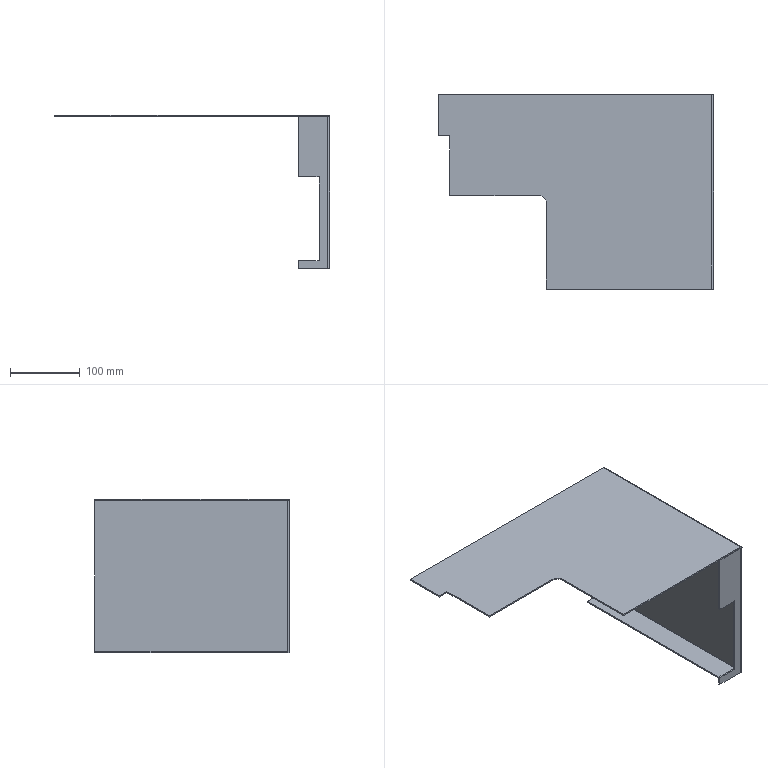Part | STEP file | TX-003 | 1 solid | 33 faces | box 395 x 279 x 220.81 mm | volume 327084 mm3 | plane 26 | cylinder 7 | commonest cylinder face diameters 1 x3 5 x3 20 x1
STEP:
#1=CARTESIAN_POINT('',(-54.654,279.925,0.));
#2=VERTEX_POINT('',#1);
#3=CARTESIAN_POINT('',(-44.654,269.925,0.));
#4=VERTEX_POINT('',#3);
#5=CARTESIAN_POINT('',(-54.654,269.925,0.));
#6=DIRECTION('',(0.,0.,-1.));
#7=DIRECTION('',(-1.,0.,0.));
#8=AXIS2_PLACEMENT_3D('',#5,#6,#7);
#9=CIRCLE('',#8,10.);
#10=EDGE_CURVE('',#2,#4,#9,.T.);
#11=ORIENTED_EDGE('',*,*,#10,.T.);
#12=CARTESIAN_POINT('',(-44.654,145.925,0.));
#13=VERTEX_POINT('',#12);
#14=CARTESIAN_POINT('',(-44.654,0.,0.));
#15=DIRECTION('',(0.,-1.,0.));
#16=VECTOR('',#15,1000.);
#17=LINE('',#14,#16);
#18=EDGE_CURVE('',#4,#13,#17,.T.);
#19=ORIENTED_EDGE('',*,*,#18,.T.);
#20=CARTESIAN_POINT('',(192.846,145.925,0.));
#21=VERTEX_POINT('',#20);
#22=CARTESIAN_POINT('',(0.,145.925,0.));
#23=DIRECTION('',(1.,0.,0.));
#24=VECTOR('',#23,1000.);
#25=LINE('',#22,#24);
#26=EDGE_CURVE('',#13,#21,#25,.T.);
#27=ORIENTED_EDGE('',*,*,#26,.T.);
#28=CARTESIAN_POINT('',(192.846,424.925,0.));
#29=VERTEX_POINT('',#28);
#30=CARTESIAN_POINT('',(192.846,0.,0.));
#31=DIRECTION('',(0.,1.,0.));
#32=VECTOR('',#31,1000.);
#33=LINE('',#30,#32);
#34=EDGE_CURVE('',#21,#29,#33,.T.);
#35=ORIENTED_EDGE('',*,*,#34,.T.);
#36=CARTESIAN_POINT('',(-199.654,424.925,0.));
#37=VERTEX_POINT('',#36);
#38=CARTESIAN_POINT('',(0.,424.925,0.));
#39=DIRECTION('',(-1.,0.,0.));
#40=VECTOR('',#39,1000.);
#41=LINE('',#38,#40);
#42=EDGE_CURVE('',#29,#37,#41,.T.);
#43=ORIENTED_EDGE('',*,*,#42,.T.);
#44=CARTESIAN_POINT('',(-199.654,365.925,0.));
#45=VERTEX_POINT('',#44);
#46=CARTESIAN_POINT('',(-199.654,0.,0.));
#47=DIRECTION('',(0.,-1.,0.));
#48=VECTOR('',#47,1000.);
#49=LINE('',#46,#48);
#50=EDGE_CURVE('',#37,#45,#49,.T.);
#51=ORIENTED_EDGE('',*,*,#50,.T.);
#52=CARTESIAN_POINT('',(-183.654,365.925,0.));
#53=VERTEX_POINT('',#52);
#54=CARTESIAN_POINT('',(0.,365.925,0.));
#55=DIRECTION('',(1.,0.,0.));
#56=VECTOR('',#55,1000.);
#57=LINE('',#54,#56);
#58=EDGE_CURVE('',#45,#53,#57,.T.);
#59=ORIENTED_EDGE('',*,*,#58,.T.);
#60=CARTESIAN_POINT('',(-183.654,279.925,0.));
#61=VERTEX_POINT('',#60);
#62=CARTESIAN_POINT('',(-183.654,0.,0.));
#63=DIRECTION('',(0.,-1.,0.));
#64=VECTOR('',#63,1000.);
#65=LINE('',#62,#64);
#66=EDGE_CURVE('',#53,#61,#65,.T.);
#67=ORIENTED_EDGE('',*,*,#66,.T.);
#68=CARTESIAN_POINT('',(0.,279.925,0.));
#69=DIRECTION('',(1.,0.,0.));
#70=VECTOR('',#69,1000.);
#71=LINE('',#68,#70);
#72=EDGE_CURVE('',#61,#2,#71,.T.);
#73=ORIENTED_EDGE('',*,*,#72,.T.);
#74=EDGE_LOOP('',(#11,#19,#27,#35,#43,#51,#59,#67,#73));
#75=FACE_OUTER_BOUND('',#74,.T.);
#76=CARTESIAN_POINT('',(0.,0.,0.));
#77=DIRECTION('',(0.,0.,1.));
#78=DIRECTION('',(1.,0.,0.));
#79=AXIS2_PLACEMENT_3D('',#76,#77,#78);
#80=PLANE('',#79);
#81=ADVANCED_FACE('',(#75),#80,.T.);
#82=CARTESIAN_POINT('',(-44.654,269.925,-2.));
#83=VERTEX_POINT('',#82);
#84=CARTESIAN_POINT('',(-44.654,145.925,-2.));
#85=VERTEX_POINT('',#84);
#86=CARTESIAN_POINT('',(-44.654,279.925,-2.));
#87=DIRECTION('',(0.,-1.,0.));
#88=VECTOR('',#87,1000.);
#89=LINE('',#86,#88);
#90=EDGE_CURVE('',#83,#85,#89,.T.);
#91=ORIENTED_EDGE('',*,*,#90,.T.);
#92=CARTESIAN_POINT('',(-44.654,145.925,-2.));
#93=DIRECTION('',(0.,0.,1.));
#94=VECTOR('',#93,1000.);
#95=LINE('',#92,#94);
#96=EDGE_CURVE('',#85,#13,#95,.T.);
#97=ORIENTED_EDGE('',*,*,#96,.T.);
#98=ORIENTED_EDGE('',*,*,#18,.F.);
#99=CARTESIAN_POINT('',(-44.654,269.925,-2.));
#100=DIRECTION('',(0.,0.,-1.));
#101=VECTOR('',#100,1000.);
#102=LINE('',#99,#101);
#103=EDGE_CURVE('',#4,#83,#102,.T.);
#104=ORIENTED_EDGE('',*,*,#103,.T.);
#105=EDGE_LOOP('',(#91,#97,#98,#104));
#106=FACE_OUTER_BOUND('',#105,.T.);
#107=CARTESIAN_POINT('',(-44.654,279.925,-2.));
#108=DIRECTION('',(-1.,0.,0.));
#109=DIRECTION('',(0.,0.,1.));
#110=AXIS2_PLACEMENT_3D('',#107,#108,#109);
#111=PLANE('',#110);
#112=ADVANCED_FACE('',(#106),#111,.T.);
#113=ORIENTED_EDGE('',*,*,#103,.F.);
#114=ORIENTED_EDGE('',*,*,#10,.F.);
#115=CARTESIAN_POINT('',(-54.654,279.925,-2.));
#116=VERTEX_POINT('',#115);
#117=CARTESIAN_POINT('',(-54.654,279.925,-2.));
#118=DIRECTION('',(0.,0.,1.));
#119=VECTOR('',#118,1000.);
#120=LINE('',#117,#119);
#121=EDGE_CURVE('',#116,#2,#120,.T.);
#122=ORIENTED_EDGE('',*,*,#121,.F.);
#123=CARTESIAN_POINT('',(-54.654,269.925,-2.));
#124=DIRECTION('',(0.,0.,1.));
#125=DIRECTION('',(-1.,0.,0.));
#126=AXIS2_PLACEMENT_3D('',#123,#124,#125);
#127=CIRCLE('',#126,10.);
#128=EDGE_CURVE('',#83,#116,#127,.T.);
#129=ORIENTED_EDGE('',*,*,#128,.F.);
#130=EDGE_LOOP('',(#113,#114,#122,#129));
#131=FACE_OUTER_BOUND('',#130,.T.);
#132=CARTESIAN_POINT('',(-54.654,269.925,-2.));
#133=DIRECTION('',(0.,0.,-1.));
#134=DIRECTION('',(-1.,0.,0.));
#135=AXIS2_PLACEMENT_3D('',#132,#133,#134);
#136=CYLINDRICAL_SURFACE('',#135,10.);
#137=ADVANCED_FACE('',(#131),#136,.F.);
#138=ORIENTED_EDGE('',*,*,#72,.F.);
#139=CARTESIAN_POINT('',(-183.654,279.925,-2.));
#140=VERTEX_POINT('',#139);
#141=CARTESIAN_POINT('',(-183.654,279.925,-2.));
#142=DIRECTION('',(0.,0.,-1.));
#143=VECTOR('',#142,1000.);
#144=LINE('',#141,#143);
#145=EDGE_CURVE('',#61,#140,#144,.T.);
#146=ORIENTED_EDGE('',*,*,#145,.T.);
#147=CARTESIAN_POINT('',(-183.654,279.925,-2.));
#148=DIRECTION('',(1.,0.,0.));
#149=VECTOR('',#148,1000.);
#150=LINE('',#147,#149);
#151=EDGE_CURVE('',#140,#116,#150,.T.);
#152=ORIENTED_EDGE('',*,*,#151,.T.);
#153=ORIENTED_EDGE('',*,*,#121,.T.);
#154=EDGE_LOOP('',(#138,#146,#152,#153));
#155=FACE_OUTER_BOUND('',#154,.T.);
#156=CARTESIAN_POINT('',(-183.654,279.925,-2.));
#157=DIRECTION('',(0.,-1.,0.));
#158=DIRECTION('',(0.,0.,-1.));
#159=AXIS2_PLACEMENT_3D('',#156,#157,#158);
#160=PLANE('',#159);
#161=ADVANCED_FACE('',(#155),#160,.T.);
#162=CARTESIAN_POINT('',(-183.654,365.925,-2.));
#163=VERTEX_POINT('',#162);
#164=CARTESIAN_POINT('',(-183.654,365.925,-2.));
#165=DIRECTION('',(0.,-1.,0.));
#166=VECTOR('',#165,1000.);
#167=LINE('',#164,#166);
#168=EDGE_CURVE('',#163,#140,#167,.T.);
#169=ORIENTED_EDGE('',*,*,#168,.T.);
#170=ORIENTED_EDGE('',*,*,#145,.F.);
#171=ORIENTED_EDGE('',*,*,#66,.F.);
#172=CARTESIAN_POINT('',(-183.654,365.925,-2.));
#173=DIRECTION('',(0.,0.,-1.));
#174=VECTOR('',#173,1000.);
#175=LINE('',#172,#174);
#176=EDGE_CURVE('',#53,#163,#175,.T.);
#177=ORIENTED_EDGE('',*,*,#176,.T.);
#178=EDGE_LOOP('',(#169,#170,#171,#177));
#179=FACE_OUTER_BOUND('',#178,.T.);
#180=CARTESIAN_POINT('',(-183.654,365.925,-2.));
#181=DIRECTION('',(-1.,0.,0.));
#182=DIRECTION('',(0.,0.,1.));
#183=AXIS2_PLACEMENT_3D('',#180,#181,#182);
#184=PLANE('',#183);
#185=ADVANCED_FACE('',(#179),#184,.T.);
#186=CARTESIAN_POINT('',(-199.654,365.925,-2.));
#187=VERTEX_POINT('',#186);
#188=CARTESIAN_POINT('',(-199.654,365.925,-2.));
#189=DIRECTION('',(1.,0.,0.));
#190=VECTOR('',#189,1000.);
#191=LINE('',#188,#190);
#192=EDGE_CURVE('',#187,#163,#191,.T.);
#193=ORIENTED_EDGE('',*,*,#192,.T.);
#194=ORIENTED_EDGE('',*,*,#176,.F.);
#195=ORIENTED_EDGE('',*,*,#58,.F.);
#196=CARTESIAN_POINT('',(-199.654,365.925,-2.));
#197=DIRECTION('',(0.,0.,-1.));
#198=VECTOR('',#197,1000.);
#199=LINE('',#196,#198);
#200=EDGE_CURVE('',#45,#187,#199,.T.);
#201=ORIENTED_EDGE('',*,*,#200,.T.);
#202=EDGE_LOOP('',(#193,#194,#195,#201));
#203=FACE_OUTER_BOUND('',#202,.T.);
#204=CARTESIAN_POINT('',(-199.654,365.925,-2.));
#205=DIRECTION('',(0.,-1.,0.));
#206=DIRECTION('',(0.,0.,-1.));
#207=AXIS2_PLACEMENT_3D('',#204,#205,#206);
#208=PLANE('',#207);
#209=ADVANCED_FACE('',(#203),#208,.T.);
#210=CARTESIAN_POINT('',(-199.654,424.925,-2.));
#211=VERTEX_POINT('',#210);
#212=CARTESIAN_POINT('',(-199.654,424.925,-2.));
#213=DIRECTION('',(0.,-1.,0.));
#214=VECTOR('',#213,1000.);
#215=LINE('',#212,#214);
#216=EDGE_CURVE('',#211,#187,#215,.T.);
#217=ORIENTED_EDGE('',*,*,#216,.T.);
#218=ORIENTED_EDGE('',*,*,#200,.F.);
#219=ORIENTED_EDGE('',*,*,#50,.F.);
#220=CARTESIAN_POINT('',(-199.654,424.925,-2.));
#221=DIRECTION('',(0.,0.,-1.));
#222=VECTOR('',#221,1000.);
#223=LINE('',#220,#222);
#224=EDGE_CURVE('',#37,#211,#223,.T.);
#225=ORIENTED_EDGE('',*,*,#224,.T.);
#226=EDGE_LOOP('',(#217,#218,#219,#225));
#227=FACE_OUTER_BOUND('',#226,.T.);
#228=CARTESIAN_POINT('',(-199.654,424.925,-2.));
#229=DIRECTION('',(-1.,0.,0.));
#230=DIRECTION('',(0.,0.,1.));
#231=AXIS2_PLACEMENT_3D('',#228,#229,#230);
#232=PLANE('',#231);
#233=ADVANCED_FACE('',(#227),#232,.T.);
#234=ORIENTED_EDGE('',*,*,#224,.F.);
#235=ORIENTED_EDGE('',*,*,#42,.F.);
#236=CARTESIAN_POINT('',(195.346,424.925,-2.5));
#237=VERTEX_POINT('',#236);
#238=CARTESIAN_POINT('',(192.846,424.925,-2.5));
#239=DIRECTION('',(0.,-1.,0.));
#240=DIRECTION('',(0.,0.,-1.));
#241=AXIS2_PLACEMENT_3D('',#238,#239,#240);
#242=CIRCLE('',#241,2.5);
#243=EDGE_CURVE('',#237,#29,#242,.T.);
#244=ORIENTED_EDGE('',*,*,#243,.F.);
#245=CARTESIAN_POINT('',(195.346,424.925,-218.31));
#246=VERTEX_POINT('',#245);
#247=CARTESIAN_POINT('',(195.346,424.925,0.));
#248=DIRECTION('',(0.,0.,1.));
#249=VECTOR('',#248,1000.);
#250=LINE('',#247,#249);
#251=EDGE_CURVE('',#246,#237,#250,.T.);
#252=ORIENTED_EDGE('',*,*,#251,.F.);
#253=CARTESIAN_POINT('',(192.846,424.925,-220.81));
#254=VERTEX_POINT('',#253);
#255=CARTESIAN_POINT('',(192.846,424.925,-218.31));
#256=DIRECTION('',(0.,-1.,0.));
#257=DIRECTION('',(0.,0.,-1.));
#258=AXIS2_PLACEMENT_3D('',#255,#256,#257);
#259=CIRCLE('',#258,2.5);
#260=EDGE_CURVE('',#254,#246,#259,.T.);
#261=ORIENTED_EDGE('',*,*,#260,.F.);
#262=CARTESIAN_POINT('',(160.346,424.925,-220.81));
#263=VERTEX_POINT('',#262);
#264=CARTESIAN_POINT('',(0.,424.925,-220.81));
#265=DIRECTION('',(1.,0.,0.));
#266=VECTOR('',#265,1000.);
#267=LINE('',#264,#266);
#268=EDGE_CURVE('',#263,#254,#267,.T.);
#269=ORIENTED_EDGE('',*,*,#268,.F.);
#270=CARTESIAN_POINT('',(160.346,424.925,-218.81));
#271=VERTEX_POINT('',#270);
#272=CARTESIAN_POINT('',(160.346,424.925,-220.81));
#273=DIRECTION('',(0.,0.,1.));
#274=VECTOR('',#273,1000.);
#275=LINE('',#272,#274);
#276=EDGE_CURVE('',#263,#271,#275,.T.);
#277=ORIENTED_EDGE('',*,*,#276,.T.);
#278=CARTESIAN_POINT('',(192.846,424.925,-218.81));
#279=VERTEX_POINT('',#278);
#280=CARTESIAN_POINT('',(160.346,424.925,-218.81));
#281=DIRECTION('',(1.,0.,0.));
#282=VECTOR('',#281,1000.);
#283=LINE('',#280,#282);
#284=EDGE_CURVE('',#271,#279,#283,.T.);
#285=ORIENTED_EDGE('',*,*,#284,.T.);
#286=CARTESIAN_POINT('',(193.346,424.925,-218.31));
#287=VERTEX_POINT('',#286);
#288=CARTESIAN_POINT('',(192.846,424.925,-218.31));
#289=DIRECTION('',(0.,-1.,0.));
#290=DIRECTION('',(0.,0.,-1.));
#291=AXIS2_PLACEMENT_3D('',#288,#289,#290);
#292=CIRCLE('',#291,0.5);
#293=EDGE_CURVE('',#279,#287,#292,.T.);
#294=ORIENTED_EDGE('',*,*,#293,.T.);
#295=CARTESIAN_POINT('',(193.346,424.925,-2.5));
#296=VERTEX_POINT('',#295);
#297=CARTESIAN_POINT('',(193.346,424.925,-220.81));
#298=DIRECTION('',(0.,0.,1.));
#299=VECTOR('',#298,1000.);
#300=LINE('',#297,#299);
#301=EDGE_CURVE('',#287,#296,#300,.T.);
#302=ORIENTED_EDGE('',*,*,#301,.T.);
#303=CARTESIAN_POINT('',(192.846,424.925,-2.));
#304=VERTEX_POINT('',#303);
#305=CARTESIAN_POINT('',(192.846,424.925,-2.5));
#306=DIRECTION('',(0.,-1.,0.));
#307=DIRECTION('',(0.,0.,-1.));
#308=AXIS2_PLACEMENT_3D('',#305,#306,#307);
#309=CIRCLE('',#308,0.5);
#310=EDGE_CURVE('',#296,#304,#309,.T.);
#311=ORIENTED_EDGE('',*,*,#310,.T.);
#312=CARTESIAN_POINT('',(-199.654,424.925,-2.));
#313=DIRECTION('',(-1.,0.,0.));
#314=VECTOR('',#313,1000.);
#315=LINE('',#312,#314);
#316=EDGE_CURVE('',#304,#211,#315,.T.);
#317=ORIENTED_EDGE('',*,*,#316,.T.);
#318=EDGE_LOOP('',(#234,#235,#244,#252,#261,#269,#277,#285,#294,#302,#311,#317));
#319=FACE_OUTER_BOUND('',#318,.T.);
#320=CARTESIAN_POINT('',(-199.654,424.925,-2.));
#321=DIRECTION('',(0.,1.,0.));
#322=DIRECTION('',(-1.,0.,0.));
#323=AXIS2_PLACEMENT_3D('',#320,#321,#322);
#324=PLANE('',#323);
#325=ADVANCED_FACE('',(#319),#324,.T.);
#326=CARTESIAN_POINT('',(195.346,148.425,-2.5));
#327=VERTEX_POINT('',#326);
#328=CARTESIAN_POINT('',(195.346,145.925,-2.5));
#329=DIRECTION('',(0.,1.,0.));
#330=VECTOR('',#329,1000.);
#331=LINE('',#328,#330);
#332=EDGE_CURVE('',#327,#237,#331,.T.);
#333=ORIENTED_EDGE('',*,*,#332,.T.);
#334=ORIENTED_EDGE('',*,*,#243,.T.);
#335=ORIENTED_EDGE('',*,*,#34,.F.);
#336=CARTESIAN_POINT('',(195.346,145.925,-2.5));
#337=VERTEX_POINT('',#336);
#338=CARTESIAN_POINT('',(192.846,145.925,-2.5));
#339=DIRECTION('',(0.,1.,0.));
#340=DIRECTION('',(0.,0.,-1.));
#341=AXIS2_PLACEMENT_3D('',#338,#339,#340);
#342=CIRCLE('',#341,2.5);
#343=EDGE_CURVE('',#21,#337,#342,.T.);
#344=ORIENTED_EDGE('',*,*,#343,.T.);
#345=CARTESIAN_POINT('',(195.346,145.925,-2.5));
#346=DIRECTION('',(0.,1.,0.));
#347=VECTOR('',#346,1000.);
#348=LINE('',#345,#347);
#349=EDGE_CURVE('',#337,#327,#348,.T.);
#350=ORIENTED_EDGE('',*,*,#349,.T.);
#351=EDGE_LOOP('',(#333,#334,#335,#344,#350));
#352=FACE_OUTER_BOUND('',#351,.T.);
#353=CARTESIAN_POINT('',(192.846,145.925,-2.5));
#354=DIRECTION('',(0.,-1.,0.));
#355=DIRECTION('',(0.,0.,-1.));
#356=AXIS2_PLACEMENT_3D('',#353,#354,#355);
#357=CYLINDRICAL_SURFACE('',#356,2.5);
#358=ADVANCED_FACE('',(#352),#357,.T.);
#359=ORIENTED_EDGE('',*,*,#26,.F.);
#360=ORIENTED_EDGE('',*,*,#96,.F.);
#361=CARTESIAN_POINT('',(192.846,145.925,-2.));
#362=VERTEX_POINT('',#361);
#363=CARTESIAN_POINT('',(-44.654,145.925,-2.));
#364=DIRECTION('',(1.,0.,0.));
#365=VECTOR('',#364,1000.);
#366=LINE('',#363,#365);
#367=EDGE_CURVE('',#85,#362,#366,.T.);
#368=ORIENTED_EDGE('',*,*,#367,.T.);
#369=CARTESIAN_POINT('',(193.346,145.925,-2.5));
#370=VERTEX_POINT('',#369);
#371=CARTESIAN_POINT('',(192.846,145.925,-2.5));
#372=DIRECTION('',(0.,-1.,0.));
#373=DIRECTION('',(0.,0.,-1.));
#374=AXIS2_PLACEMENT_3D('',#371,#372,#373);
#375=CIRCLE('',#374,0.5);
#376=EDGE_CURVE('',#370,#362,#375,.T.);
#377=ORIENTED_EDGE('',*,*,#376,.F.);
#378=CARTESIAN_POINT('',(193.346,145.925,-2.5));
#379=DIRECTION('',(-1.,0.,0.));
#380=VECTOR('',#379,1000.);
#381=LINE('',#378,#380);
#382=EDGE_CURVE('',#337,#370,#381,.T.);
#383=ORIENTED_EDGE('',*,*,#382,.F.);
#384=ORIENTED_EDGE('',*,*,#343,.F.);
#385=EDGE_LOOP('',(#359,#360,#368,#377,#383,#384));
#386=FACE_OUTER_BOUND('',#385,.T.);
#387=CARTESIAN_POINT('',(-44.654,145.925,-2.));
#388=DIRECTION('',(0.,-1.,0.));
#389=DIRECTION('',(1.,0.,0.));
#390=AXIS2_PLACEMENT_3D('',#387,#388,#389);
#391=PLANE('',#390);
#392=ADVANCED_FACE('',(#386),#391,.T.);
#393=ORIENTED_EDGE('',*,*,#367,.F.);
#394=ORIENTED_EDGE('',*,*,#90,.F.);
#395=ORIENTED_EDGE('',*,*,#128,.T.);
#396=ORIENTED_EDGE('',*,*,#151,.F.);
#397=ORIENTED_EDGE('',*,*,#168,.F.);
#398=ORIENTED_EDGE('',*,*,#192,.F.);
#399=ORIENTED_EDGE('',*,*,#216,.F.);
#400=ORIENTED_EDGE('',*,*,#316,.F.);
#401=CARTESIAN_POINT('',(192.846,0.,-2.));
#402=DIRECTION('',(0.,1.,0.));
#403=VECTOR('',#402,1000.);
#404=LINE('',#401,#403);
#405=EDGE_CURVE('',#362,#304,#404,.T.);
#406=ORIENTED_EDGE('',*,*,#405,.F.);
#407=EDGE_LOOP('',(#393,#394,#395,#396,#397,#398,#399,#400,#406));
#408=FACE_OUTER_BOUND('',#407,.T.);
#409=CARTESIAN_POINT('',(0.,0.,-2.));
#410=DIRECTION('',(0.,0.,1.));
#411=DIRECTION('',(1.,0.,0.));
#412=AXIS2_PLACEMENT_3D('',#409,#410,#411);
#413=PLANE('',#412);
#414=ADVANCED_FACE('',(#408),#413,.F.);
#415=ORIENTED_EDGE('',*,*,#251,.T.);
#416=ORIENTED_EDGE('',*,*,#332,.F.);
#417=CARTESIAN_POINT('',(195.346,148.425,-218.31));
#418=VERTEX_POINT('',#417);
#419=CARTESIAN_POINT('',(195.346,148.425,0.));
#420=DIRECTION('',(0.,0.,-1.));
#421=VECTOR('',#420,1000.);
#422=LINE('',#419,#421);
#423=EDGE_CURVE('',#327,#418,#422,.T.);
#424=ORIENTED_EDGE('',*,*,#423,.T.);
#425=CARTESIAN_POINT('',(195.346,0.,-218.31));
#426=DIRECTION('',(0.,1.,0.));
#427=VECTOR('',#426,1000.);
#428=LINE('',#425,#427);
#429=EDGE_CURVE('',#418,#246,#428,.T.);
#430=ORIENTED_EDGE('',*,*,#429,.T.);
#431=EDGE_LOOP('',(#415,#416,#424,#430));
#432=FACE_OUTER_BOUND('',#431,.T.);
#433=CARTESIAN_POINT('',(195.346,0.,0.));
#434=DIRECTION('',(1.,0.,0.));
#435=DIRECTION('',(0.,0.,-1.));
#436=AXIS2_PLACEMENT_3D('',#433,#434,#435);
#437=PLANE('',#436);
#438=ADVANCED_FACE('',(#432),#437,.T.);
#439=ORIENTED_EDGE('',*,*,#349,.F.);
#440=ORIENTED_EDGE('',*,*,#382,.T.);
#441=CARTESIAN_POINT('',(193.346,145.975,-2.5));
#442=VERTEX_POINT('',#441);
#443=CARTESIAN_POINT('',(193.346,145.925,-2.5));
#444=DIRECTION('',(0.,1.,0.));
#445=VECTOR('',#444,1000.);
#446=LINE('',#443,#445);
#447=EDGE_CURVE('',#370,#442,#446,.T.);
#448=ORIENTED_EDGE('',*,*,#447,.T.);
#449=CARTESIAN_POINT('',(192.846,148.425,-2.5));
#450=DIRECTION('',(0.,0.,1.));
#451=DIRECTION('',(1.,0.,0.));
#452=AXIS2_PLACEMENT_3D('',#449,#450,#451);
#453=CIRCLE('',#452,2.5);
#454=EDGE_CURVE('',#442,#327,#453,.T.);
#455=ORIENTED_EDGE('',*,*,#454,.T.);
#456=EDGE_LOOP('',(#439,#440,#448,#455));
#457=FACE_OUTER_BOUND('',#456,.T.);
#458=CARTESIAN_POINT('',(193.346,145.925,-2.5));
#459=DIRECTION('',(0.,0.,-1.));
#460=DIRECTION('',(-1.,0.,0.));
#461=AXIS2_PLACEMENT_3D('',#458,#459,#460);
#462=PLANE('',#461);
#463=ADVANCED_FACE('',(#457),#462,.T.);
#464=ORIENTED_EDGE('',*,*,#310,.F.);
#465=CARTESIAN_POINT('',(193.346,148.425,-2.5));
#466=VERTEX_POINT('',#465);
#467=CARTESIAN_POINT('',(193.346,145.925,-2.5));
#468=DIRECTION('',(0.,1.,0.));
#469=VECTOR('',#468,1000.);
#470=LINE('',#467,#469);
#471=EDGE_CURVE('',#466,#296,#470,.T.);
#472=ORIENTED_EDGE('',*,*,#471,.F.);
#473=CARTESIAN_POINT('',(193.346,145.925,-2.5));
#474=DIRECTION('',(0.,1.,0.));
#475=VECTOR('',#474,1000.);
#476=LINE('',#473,#475);
#477=EDGE_CURVE('',#442,#466,#476,.T.);
#478=ORIENTED_EDGE('',*,*,#477,.F.);
#479=ORIENTED_EDGE('',*,*,#447,.F.);
#480=ORIENTED_EDGE('',*,*,#376,.T.);
#481=ORIENTED_EDGE('',*,*,#405,.T.);
#482=EDGE_LOOP('',(#464,#472,#478,#479,#480,#481));
#483=FACE_OUTER_BOUND('',#482,.T.);
#484=CARTESIAN_POINT('',(192.846,145.925,-2.5));
#485=DIRECTION('',(0.,-1.,0.));
#486=DIRECTION('',(0.,0.,-1.));
#487=AXIS2_PLACEMENT_3D('',#484,#485,#486);
#488=CYLINDRICAL_SURFACE('',#487,0.5);
#489=ADVANCED_FACE('',(#483),#488,.F.);
#490=CARTESIAN_POINT('',(192.846,148.425,-220.81));
#491=VERTEX_POINT('',#490);
#492=CARTESIAN_POINT('',(192.846,148.425,-220.81));
#493=DIRECTION('',(0.,1.,0.));
#494=VECTOR('',#493,1000.);
#495=LINE('',#492,#494);
#496=EDGE_CURVE('',#491,#254,#495,.T.);
#497=ORIENTED_EDGE('',*,*,#496,.T.);
#498=ORIENTED_EDGE('',*,*,#260,.T.);
#499=ORIENTED_EDGE('',*,*,#429,.F.);
#500=CARTESIAN_POINT('',(193.346,148.425,-220.759));
#501=VERTEX_POINT('',#500);
#502=CARTESIAN_POINT('',(192.846,148.425,-218.31));
#503=DIRECTION('',(0.,1.,0.));
#504=DIRECTION('',(0.,0.,-1.));
#505=AXIS2_PLACEMENT_3D('',#502,#503,#504);
#506=CIRCLE('',#505,2.5);
#507=EDGE_CURVE('',#418,#501,#506,.T.);
#508=ORIENTED_EDGE('',*,*,#507,.T.);
#509=CARTESIAN_POINT('',(192.846,148.425,-218.31));
#510=DIRECTION('',(0.,1.,0.));
#511=DIRECTION('',(0.,0.,-1.));
#512=AXIS2_PLACEMENT_3D('',#509,#510,#511);
#513=CIRCLE('',#512,2.5);
#514=EDGE_CURVE('',#501,#491,#513,.T.);
#515=ORIENTED_EDGE('',*,*,#514,.T.);
#516=EDGE_LOOP('',(#497,#498,#499,#508,#515));
#517=FACE_OUTER_BOUND('',#516,.T.);
#518=CARTESIAN_POINT('',(192.846,148.425,-218.31));
#519=DIRECTION('',(0.,-1.,0.));
#520=DIRECTION('',(0.,0.,-1.));
#521=AXIS2_PLACEMENT_3D('',#518,#519,#520);
#522=CYLINDRICAL_SURFACE('',#521,2.5);
#523=ADVANCED_FACE('',(#517),#522,.T.);
#524=CARTESIAN_POINT('',(192.846,145.925,-220.81));
#525=VERTEX_POINT('',#524);
#526=CARTESIAN_POINT('',(195.346,148.425,-220.81));
#527=VERTEX_POINT('',#526);
#528=CARTESIAN_POINT('',(192.846,148.425,-220.81));
#529=DIRECTION('',(0.,0.,1.));
#530=DIRECTION('',(1.,0.,0.));
#531=AXIS2_PLACEMENT_3D('',#528,#529,#530);
#532=CIRCLE('',#531,2.5);
#533=EDGE_CURVE('',#525,#527,#532,.T.);
#534=ORIENTED_EDGE('',*,*,#533,.T.);
#535=CARTESIAN_POINT('',(195.346,148.425,-2.5));
#536=DIRECTION('',(0.,0.,1.));
#537=VECTOR('',#536,1000.);
#538=LINE('',#535,#537);
#539=EDGE_CURVE('',#527,#418,#538,.T.);
#540=ORIENTED_EDGE('',*,*,#539,.T.);
#541=ORIENTED_EDGE('',*,*,#423,.F.);
#542=ORIENTED_EDGE('',*,*,#454,.F.);
#543=CARTESIAN_POINT('',(192.846,145.925,-2.5));
#544=VERTEX_POINT('',#543);
#545=CARTESIAN_POINT('',(192.846,148.425,-2.5));
#546=DIRECTION('',(0.,0.,-1.));
#547=DIRECTION('',(1.,0.,0.));
#548=AXIS2_PLACEMENT_3D('',#545,#546,#547);
#549=CIRCLE('',#548,2.5);
#550=EDGE_CURVE('',#442,#544,#549,.T.);
#551=ORIENTED_EDGE('',*,*,#550,.T.);
#552=CARTESIAN_POINT('',(192.846,145.925,-2.5));
#553=DIRECTION('',(0.,0.,-1.));
#554=VECTOR('',#553,1000.);
#555=LINE('',#552,#554);
#556=EDGE_CURVE('',#544,#525,#555,.T.);
#557=ORIENTED_EDGE('',*,*,#556,.T.);
#558=EDGE_LOOP('',(#534,#540,#541,#542,#551,#557));
#559=FACE_OUTER_BOUND('',#558,.T.);
#560=CARTESIAN_POINT('',(192.846,148.425,-2.5));
#561=DIRECTION('',(0.,0.,1.));
#562=DIRECTION('',(1.,0.,0.));
#563=AXIS2_PLACEMENT_3D('',#560,#561,#562);
#564=CYLINDRICAL_SURFACE('',#563,2.5);
#565=ADVANCED_FACE('',(#559),#564,.T.);
#566=CARTESIAN_POINT('',(193.346,148.425,-218.31));
#567=VERTEX_POINT('',#566);
#568=CARTESIAN_POINT('',(193.346,148.425,0.));
#569=DIRECTION('',(0.,0.,-1.));
#570=VECTOR('',#569,1000.);
#571=LINE('',#568,#570);
#572=EDGE_CURVE('',#466,#567,#571,.T.);
#573=ORIENTED_EDGE('',*,*,#572,.F.);
#574=ORIENTED_EDGE('',*,*,#471,.T.);
#575=ORIENTED_EDGE('',*,*,#301,.F.);
#576=CARTESIAN_POINT('',(193.346,0.,-218.31));
#577=DIRECTION('',(0.,1.,0.));
#578=VECTOR('',#577,1000.);
#579=LINE('',#576,#578);
#580=EDGE_CURVE('',#567,#287,#579,.T.);
#581=ORIENTED_EDGE('',*,*,#580,.F.);
#582=EDGE_LOOP('',(#573,#574,#575,#581));
#583=FACE_OUTER_BOUND('',#582,.T.);
#584=CARTESIAN_POINT('',(193.346,0.,0.));
#585=DIRECTION('',(1.,0.,0.));
#586=DIRECTION('',(0.,0.,-1.));
#587=AXIS2_PLACEMENT_3D('',#584,#585,#586);
#588=PLANE('',#587);
#589=ADVANCED_FACE('',(#583),#588,.F.);
#590=ORIENTED_EDGE('',*,*,#477,.T.);
#591=CARTESIAN_POINT('',(192.846,147.925,-2.5));
#592=VERTEX_POINT('',#591);
#593=CARTESIAN_POINT('',(192.846,148.425,-2.5));
#594=DIRECTION('',(0.,0.,1.));
#595=DIRECTION('',(1.,0.,0.));
#596=AXIS2_PLACEMENT_3D('',#593,#594,#595);
#597=CIRCLE('',#596,0.5);
#598=EDGE_CURVE('',#592,#466,#597,.T.);
#599=ORIENTED_EDGE('',*,*,#598,.F.);
#600=CARTESIAN_POINT('',(150.346,147.925,-2.5));
#601=VERTEX_POINT('',#600);
#602=CARTESIAN_POINT('',(193.346,147.925,-2.5));
#603=DIRECTION('',(-1.,0.,0.));
#604=VECTOR('',#603,1000.);
#605=LINE('',#602,#604);
#606=EDGE_CURVE('',#592,#601,#605,.T.);
#607=ORIENTED_EDGE('',*,*,#606,.T.);
#608=CARTESIAN_POINT('',(150.346,145.925,-2.5));
#609=VERTEX_POINT('',#608);
#610=CARTESIAN_POINT('',(150.346,145.925,-2.5));
#611=DIRECTION('',(0.,-1.,0.));
#612=VECTOR('',#611,1000.);
#613=LINE('',#610,#612);
#614=EDGE_CURVE('',#601,#609,#613,.T.);
#615=ORIENTED_EDGE('',*,*,#614,.T.);
#616=CARTESIAN_POINT('',(0.,145.925,-2.5));
#617=DIRECTION('',(-1.,0.,0.));
#618=VECTOR('',#617,1000.);
#619=LINE('',#616,#618);
#620=EDGE_CURVE('',#544,#609,#619,.T.);
#621=ORIENTED_EDGE('',*,*,#620,.F.);
#622=ORIENTED_EDGE('',*,*,#550,.F.);
#623=EDGE_LOOP('',(#590,#599,#607,#615,#621,#622));
#624=FACE_OUTER_BOUND('',#623,.T.);
#625=CARTESIAN_POINT('',(192.846,148.425,-2.5));
#626=DIRECTION('',(0.,0.,-1.));
#627=DIRECTION('',(-1.,0.,0.));
#628=AXIS2_PLACEMENT_3D('',#625,#626,#627);
#629=PLANE('',#628);
#630=ADVANCED_FACE('',(#624),#629,.F.);
#631=CARTESIAN_POINT('',(160.346,148.425,-220.81));
#632=VERTEX_POINT('',#631);
#633=CARTESIAN_POINT('',(0.,148.425,-220.81));
#634=DIRECTION('',(-1.,0.,0.));
#635=VECTOR('',#634,1000.);
#636=LINE('',#633,#635);
#637=EDGE_CURVE('',#491,#632,#636,.T.);
#638=ORIENTED_EDGE('',*,*,#637,.T.);
#639=CARTESIAN_POINT('',(160.346,0.,-220.81));
#640=DIRECTION('',(0.,1.,0.));
#641=VECTOR('',#640,1000.);
#642=LINE('',#639,#641);
#643=EDGE_CURVE('',#632,#263,#642,.T.);
#644=ORIENTED_EDGE('',*,*,#643,.T.);
#645=ORIENTED_EDGE('',*,*,#268,.T.);
#646=ORIENTED_EDGE('',*,*,#496,.F.);
#647=EDGE_LOOP('',(#638,#644,#645,#646));
#648=FACE_OUTER_BOUND('',#647,.T.);
#649=CARTESIAN_POINT('',(0.,0.,-220.81));
#650=DIRECTION('',(0.,0.,-1.));
#651=DIRECTION('',(-1.,0.,0.));
#652=AXIS2_PLACEMENT_3D('',#649,#650,#651);
#653=PLANE('',#652);
#654=ADVANCED_FACE('',(#648),#653,.T.);
#655=ORIENTED_EDGE('',*,*,#539,.F.);
#656=CARTESIAN_POINT('',(193.346,148.425,-220.81));
#657=VERTEX_POINT('',#656);
#658=CARTESIAN_POINT('',(193.346,148.425,-220.81));
#659=DIRECTION('',(-1.,0.,0.));
#660=VECTOR('',#659,1000.);
#661=LINE('',#658,#660);
#662=EDGE_CURVE('',#527,#657,#661,.T.);
#663=ORIENTED_EDGE('',*,*,#662,.T.);
#664=CARTESIAN_POINT('',(193.346,148.425,-220.81));
#665=DIRECTION('',(0.,0.,1.));
#666=VECTOR('',#665,1000.);
#667=LINE('',#664,#666);
#668=EDGE_CURVE('',#657,#501,#667,.T.);
#669=ORIENTED_EDGE('',*,*,#668,.T.);
#670=ORIENTED_EDGE('',*,*,#507,.F.);
#671=EDGE_LOOP('',(#655,#663,#669,#670));
#672=FACE_OUTER_BOUND('',#671,.T.);
#673=CARTESIAN_POINT('',(193.346,148.425,-220.81));
#674=DIRECTION('',(0.,1.,0.));
#675=DIRECTION('',(-1.,0.,0.));
#676=AXIS2_PLACEMENT_3D('',#673,#674,#675);
#677=PLANE('',#676);
#678=ADVANCED_FACE('',(#672),#677,.T.);
#679=ORIENTED_EDGE('',*,*,#662,.F.);
#680=ORIENTED_EDGE('',*,*,#533,.F.);
#681=CARTESIAN_POINT('',(150.346,145.925,-220.81));
#682=VERTEX_POINT('',#681);
#683=CARTESIAN_POINT('',(0.,145.925,-220.81));
#684=DIRECTION('',(1.,0.,0.));
#685=VECTOR('',#684,1000.);
#686=LINE('',#683,#685);
#687=EDGE_CURVE('',#682,#525,#686,.T.);
#688=ORIENTED_EDGE('',*,*,#687,.F.);
#689=CARTESIAN_POINT('',(150.346,147.925,-220.81));
#690=VERTEX_POINT('',#689);
#691=CARTESIAN_POINT('',(150.346,145.925,-220.81));
#692=DIRECTION('',(0.,1.,0.));
#693=VECTOR('',#692,1000.);
#694=LINE('',#691,#693);
#695=EDGE_CURVE('',#682,#690,#694,.T.);
#696=ORIENTED_EDGE('',*,*,#695,.T.);
#697=CARTESIAN_POINT('',(192.846,147.925,-220.81));
#698=VERTEX_POINT('',#697);
#699=CARTESIAN_POINT('',(150.346,147.925,-220.81));
#700=DIRECTION('',(1.,0.,0.));
#701=VECTOR('',#700,1000.);
#702=LINE('',#699,#701);
#703=EDGE_CURVE('',#690,#698,#702,.T.);
#704=ORIENTED_EDGE('',*,*,#703,.T.);
#705=CARTESIAN_POINT('',(192.846,148.425,-220.81));
#706=DIRECTION('',(0.,0.,1.));
#707=DIRECTION('',(1.,0.,0.));
#708=AXIS2_PLACEMENT_3D('',#705,#706,#707);
#709=CIRCLE('',#708,0.5);
#710=EDGE_CURVE('',#698,#657,#709,.T.);
#711=ORIENTED_EDGE('',*,*,#710,.T.);
#712=EDGE_LOOP('',(#679,#680,#688,#696,#704,#711));
#713=FACE_OUTER_BOUND('',#712,.T.);
#714=CARTESIAN_POINT('',(192.846,148.425,-220.81));
#715=DIRECTION('',(0.,0.,-1.));
#716=DIRECTION('',(-1.,0.,0.));
#717=AXIS2_PLACEMENT_3D('',#714,#715,#716);
#718=PLANE('',#717);
#719=ADVANCED_FACE('',(#713),#718,.T.);
#720=CARTESIAN_POINT('',(150.346,145.925,-88.81));
#721=VERTEX_POINT('',#720);
#722=CARTESIAN_POINT('',(180.346,145.925,-88.81));
#723=VERTEX_POINT('',#722);
#724=CARTESIAN_POINT('',(0.,145.925,-88.81));
#725=DIRECTION('',(1.,0.,0.));
#726=VECTOR('',#725,1000.);
#727=LINE('',#724,#726);
#728=EDGE_CURVE('',#721,#723,#727,.T.);
#729=ORIENTED_EDGE('',*,*,#728,.T.);
#730=CARTESIAN_POINT('',(180.346,145.925,-208.81));
#731=VERTEX_POINT('',#730);
#732=CARTESIAN_POINT('',(180.346,145.925,0.));
#733=DIRECTION('',(0.,0.,-1.));
#734=VECTOR('',#733,1000.);
#735=LINE('',#732,#734);
#736=EDGE_CURVE('',#723,#731,#735,.T.);
#737=ORIENTED_EDGE('',*,*,#736,.T.);
#738=CARTESIAN_POINT('',(150.346,145.925,-208.81));
#739=VERTEX_POINT('',#738);
#740=CARTESIAN_POINT('',(0.,145.925,-208.81));
#741=DIRECTION('',(-1.,0.,0.));
#742=VECTOR('',#741,1000.);
#743=LINE('',#740,#742);
#744=EDGE_CURVE('',#731,#739,#743,.T.);
#745=ORIENTED_EDGE('',*,*,#744,.T.);
#746=CARTESIAN_POINT('',(150.346,145.925,0.));
#747=DIRECTION('',(0.,0.,-1.));
#748=VECTOR('',#747,1000.);
#749=LINE('',#746,#748);
#750=EDGE_CURVE('',#739,#682,#749,.T.);
#751=ORIENTED_EDGE('',*,*,#750,.T.);
#752=ORIENTED_EDGE('',*,*,#687,.T.);
#753=ORIENTED_EDGE('',*,*,#556,.F.);
#754=ORIENTED_EDGE('',*,*,#620,.T.);
#755=CARTESIAN_POINT('',(150.346,145.925,0.));
#756=DIRECTION('',(0.,0.,-1.));
#757=VECTOR('',#756,1000.);
#758=LINE('',#755,#757);
#759=EDGE_CURVE('',#609,#721,#758,.T.);
#760=ORIENTED_EDGE('',*,*,#759,.T.);
#761=EDGE_LOOP('',(#729,#737,#745,#751,#752,#753,#754,#760));
#762=FACE_OUTER_BOUND('',#761,.T.);
#763=CARTESIAN_POINT('',(0.,145.925,0.));
#764=DIRECTION('',(0.,-1.,0.));
#765=DIRECTION('',(1.,0.,0.));
#766=AXIS2_PLACEMENT_3D('',#763,#764,#765);
#767=PLANE('',#766);
#768=ADVANCED_FACE('',(#762),#767,.T.);
#769=ORIENTED_EDGE('',*,*,#293,.F.);
#770=CARTESIAN_POINT('',(192.846,148.425,-218.81));
#771=VERTEX_POINT('',#770);
#772=CARTESIAN_POINT('',(192.846,148.425,-218.81));
#773=DIRECTION('',(0.,1.,0.));
#774=VECTOR('',#773,1000.);
#775=LINE('',#772,#774);
#776=EDGE_CURVE('',#771,#279,#775,.T.);
#777=ORIENTED_EDGE('',*,*,#776,.F.);
#778=CARTESIAN_POINT('',(192.846,148.425,-218.31));
#779=DIRECTION('',(0.,-1.,0.));
#780=DIRECTION('',(0.,0.,-1.));
#781=AXIS2_PLACEMENT_3D('',#778,#779,#780);
#782=CIRCLE('',#781,0.5);
#783=EDGE_CURVE('',#771,#567,#782,.T.);
#784=ORIENTED_EDGE('',*,*,#783,.T.);
#785=ORIENTED_EDGE('',*,*,#580,.T.);
#786=EDGE_LOOP('',(#769,#777,#784,#785));
#787=FACE_OUTER_BOUND('',#786,.T.);
#788=CARTESIAN_POINT('',(192.846,148.425,-218.31));
#789=DIRECTION('',(0.,-1.,0.));
#790=DIRECTION('',(0.,0.,-1.));
#791=AXIS2_PLACEMENT_3D('',#788,#789,#790);
#792=CYLINDRICAL_SURFACE('',#791,0.5);
#793=ADVANCED_FACE('',(#787),#792,.F.);
#794=CARTESIAN_POINT('',(193.346,148.425,-2.5));
#795=DIRECTION('',(0.,0.,1.));
#796=VECTOR('',#795,1000.);
#797=LINE('',#794,#796);
#798=EDGE_CURVE('',#501,#567,#797,.T.);
#799=ORIENTED_EDGE('',*,*,#798,.F.);
#800=ORIENTED_EDGE('',*,*,#668,.F.);
#801=ORIENTED_EDGE('',*,*,#710,.F.);
#802=CARTESIAN_POINT('',(192.846,147.925,-2.5));
#803=DIRECTION('',(0.,0.,-1.));
#804=VECTOR('',#803,1000.);
#805=LINE('',#802,#804);
#806=EDGE_CURVE('',#592,#698,#805,.T.);
#807=ORIENTED_EDGE('',*,*,#806,.F.);
#808=ORIENTED_EDGE('',*,*,#598,.T.);
#809=ORIENTED_EDGE('',*,*,#572,.T.);
#810=EDGE_LOOP('',(#799,#800,#801,#807,#808,#809));
#811=FACE_OUTER_BOUND('',#810,.T.);
#812=CARTESIAN_POINT('',(192.846,148.425,-2.5));
#813=DIRECTION('',(0.,0.,1.));
#814=DIRECTION('',(1.,0.,0.));
#815=AXIS2_PLACEMENT_3D('',#812,#813,#814);
#816=CYLINDRICAL_SURFACE('',#815,0.5);
#817=ADVANCED_FACE('',(#811),#816,.F.);
#818=ORIENTED_EDGE('',*,*,#643,.F.);
#819=CARTESIAN_POINT('',(160.346,148.425,-218.81));
#820=VERTEX_POINT('',#819);
#821=CARTESIAN_POINT('',(160.346,148.425,-220.81));
#822=DIRECTION('',(0.,0.,1.));
#823=VECTOR('',#822,1000.);
#824=LINE('',#821,#823);
#825=EDGE_CURVE('',#632,#820,#824,.T.);
#826=ORIENTED_EDGE('',*,*,#825,.T.);
#827=CARTESIAN_POINT('',(160.346,148.425,-218.81));
#828=DIRECTION('',(0.,1.,0.));
#829=VECTOR('',#828,1000.);
#830=LINE('',#827,#829);
#831=EDGE_CURVE('',#820,#271,#830,.T.);
#832=ORIENTED_EDGE('',*,*,#831,.T.);
#833=ORIENTED_EDGE('',*,*,#276,.F.);
#834=EDGE_LOOP('',(#818,#826,#832,#833));
#835=FACE_OUTER_BOUND('',#834,.T.);
#836=CARTESIAN_POINT('',(160.346,148.425,-220.81));
#837=DIRECTION('',(-1.,0.,0.));
#838=DIRECTION('',(0.,0.,1.));
#839=AXIS2_PLACEMENT_3D('',#836,#837,#838);
#840=PLANE('',#839);
#841=ADVANCED_FACE('',(#835),#840,.T.);
#842=CARTESIAN_POINT('',(193.346,148.425,-218.81));
#843=DIRECTION('',(-1.,0.,0.));
#844=VECTOR('',#843,1000.);
#845=LINE('',#842,#844);
#846=EDGE_CURVE('',#771,#820,#845,.T.);
#847=ORIENTED_EDGE('',*,*,#846,.T.);
#848=ORIENTED_EDGE('',*,*,#825,.F.);
#849=ORIENTED_EDGE('',*,*,#637,.F.);
#850=ORIENTED_EDGE('',*,*,#514,.F.);
#851=ORIENTED_EDGE('',*,*,#798,.T.);
#852=ORIENTED_EDGE('',*,*,#783,.F.);
#853=EDGE_LOOP('',(#847,#848,#849,#850,#851,#852));
#854=FACE_OUTER_BOUND('',#853,.T.);
#855=CARTESIAN_POINT('',(193.346,148.425,-220.81));
#856=DIRECTION('',(0.,-1.,0.));
#857=DIRECTION('',(0.,0.,-1.));
#858=AXIS2_PLACEMENT_3D('',#855,#856,#857);
#859=PLANE('',#858);
#860=ADVANCED_FACE('',(#854),#859,.T.);
#861=CARTESIAN_POINT('',(180.346,147.925,-88.81));
#862=VERTEX_POINT('',#861);
#863=CARTESIAN_POINT('',(180.346,137.925,-88.81));
#864=DIRECTION('',(0.,-1.,0.));
#865=VECTOR('',#864,1000.);
#866=LINE('',#863,#865);
#867=EDGE_CURVE('',#862,#723,#866,.T.);
#868=ORIENTED_EDGE('',*,*,#867,.F.);
#869=CARTESIAN_POINT('',(180.346,147.925,-208.81));
#870=VERTEX_POINT('',#869);
#871=CARTESIAN_POINT('',(180.346,147.925,-88.81));
#872=DIRECTION('',(0.,0.,1.));
#873=VECTOR('',#872,1000.);
#874=LINE('',#871,#873);
#875=EDGE_CURVE('',#870,#862,#874,.T.);
#876=ORIENTED_EDGE('',*,*,#875,.F.);
#877=CARTESIAN_POINT('',(180.346,137.925,-208.81));
#878=DIRECTION('',(0.,1.,0.));
#879=VECTOR('',#878,1000.);
#880=LINE('',#877,#879);
#881=EDGE_CURVE('',#731,#870,#880,.T.);
#882=ORIENTED_EDGE('',*,*,#881,.F.);
#883=ORIENTED_EDGE('',*,*,#736,.F.);
#884=EDGE_LOOP('',(#868,#876,#882,#883));
#885=FACE_OUTER_BOUND('',#884,.T.);
#886=CARTESIAN_POINT('',(180.346,137.925,-88.81));
#887=DIRECTION('',(1.,0.,0.));
#888=DIRECTION('',(0.,1.,0.));
#889=AXIS2_PLACEMENT_3D('',#886,#887,#888);
#890=PLANE('',#889);
#891=ADVANCED_FACE('',(#885),#890,.F.);
#892=CARTESIAN_POINT('',(150.346,147.925,-88.81));
#893=VERTEX_POINT('',#892);
#894=CARTESIAN_POINT('',(150.346,137.925,-88.81));
#895=DIRECTION('',(0.,-1.,0.));
#896=VECTOR('',#895,1000.);
#897=LINE('',#894,#896);
#898=EDGE_CURVE('',#893,#721,#897,.T.);
#899=ORIENTED_EDGE('',*,*,#898,.F.);
#900=CARTESIAN_POINT('',(150.346,147.925,-88.81));
#901=DIRECTION('',(-1.,0.,0.));
#902=VECTOR('',#901,1000.);
#903=LINE('',#900,#902);
#904=EDGE_CURVE('',#862,#893,#903,.T.);
#905=ORIENTED_EDGE('',*,*,#904,.F.);
#906=ORIENTED_EDGE('',*,*,#867,.T.);
#907=ORIENTED_EDGE('',*,*,#728,.F.);
#908=EDGE_LOOP('',(#899,#905,#906,#907));
#909=FACE_OUTER_BOUND('',#908,.T.);
#910=CARTESIAN_POINT('',(150.346,137.925,-88.81));
#911=DIRECTION('',(0.,0.,1.));
#912=DIRECTION('',(0.,-1.,0.));
#913=AXIS2_PLACEMENT_3D('',#910,#911,#912);
#914=PLANE('',#913);
#915=ADVANCED_FACE('',(#909),#914,.F.);
#916=ORIENTED_EDGE('',*,*,#614,.F.);
#917=CARTESIAN_POINT('',(150.346,147.925,-2.5));
#918=DIRECTION('',(0.,0.,-1.));
#919=VECTOR('',#918,1000.);
#920=LINE('',#917,#919);
#921=EDGE_CURVE('',#601,#893,#920,.T.);
#922=ORIENTED_EDGE('',*,*,#921,.T.);
#923=ORIENTED_EDGE('',*,*,#898,.T.);
#924=ORIENTED_EDGE('',*,*,#759,.F.);
#925=EDGE_LOOP('',(#916,#922,#923,#924));
#926=FACE_OUTER_BOUND('',#925,.T.);
#927=CARTESIAN_POINT('',(150.346,145.925,-2.5));
#928=DIRECTION('',(-1.,0.,0.));
#929=DIRECTION('',(0.,-1.,0.));
#930=AXIS2_PLACEMENT_3D('',#927,#928,#929);
#931=PLANE('',#930);
#932=ADVANCED_FACE('',(#926),#931,.T.);
#933=ORIENTED_EDGE('',*,*,#695,.F.);
#934=ORIENTED_EDGE('',*,*,#750,.F.);
#935=CARTESIAN_POINT('',(150.346,147.925,-208.81));
#936=VERTEX_POINT('',#935);
#937=CARTESIAN_POINT('',(150.346,145.925,-208.81));
#938=DIRECTION('',(0.,1.,0.));
#939=VECTOR('',#938,1000.);
#940=LINE('',#937,#939);
#941=EDGE_CURVE('',#739,#936,#940,.T.);
#942=ORIENTED_EDGE('',*,*,#941,.T.);
#943=CARTESIAN_POINT('',(150.346,147.925,-2.5));
#944=DIRECTION('',(0.,0.,-1.));
#945=VECTOR('',#944,1000.);
#946=LINE('',#943,#945);
#947=EDGE_CURVE('',#936,#690,#946,.T.);
#948=ORIENTED_EDGE('',*,*,#947,.T.);
#949=EDGE_LOOP('',(#933,#934,#942,#948));
#950=FACE_OUTER_BOUND('',#949,.T.);
#951=CARTESIAN_POINT('',(150.346,145.925,-2.5));
#952=DIRECTION('',(-1.,0.,0.));
#953=DIRECTION('',(0.,-1.,0.));
#954=AXIS2_PLACEMENT_3D('',#951,#952,#953);
#955=PLANE('',#954);
#956=ADVANCED_FACE('',(#950),#955,.T.);
#957=ORIENTED_EDGE('',*,*,#881,.T.);
#958=CARTESIAN_POINT('',(150.346,147.925,-208.81));
#959=DIRECTION('',(1.,0.,0.));
#960=VECTOR('',#959,1000.);
#961=LINE('',#958,#960);
#962=EDGE_CURVE('',#936,#870,#961,.T.);
#963=ORIENTED_EDGE('',*,*,#962,.F.);
#964=ORIENTED_EDGE('',*,*,#941,.F.);
#965=ORIENTED_EDGE('',*,*,#744,.F.);
#966=EDGE_LOOP('',(#957,#963,#964,#965));
#967=FACE_OUTER_BOUND('',#966,.T.);
#968=CARTESIAN_POINT('',(150.346,137.925,-208.81));
#969=DIRECTION('',(0.,0.,-1.));
#970=DIRECTION('',(0.,1.,0.));
#971=AXIS2_PLACEMENT_3D('',#968,#969,#970);
#972=PLANE('',#971);
#973=ADVANCED_FACE('',(#967),#972,.F.);
#974=ORIENTED_EDGE('',*,*,#284,.F.);
#975=ORIENTED_EDGE('',*,*,#831,.F.);
#976=ORIENTED_EDGE('',*,*,#846,.F.);
#977=ORIENTED_EDGE('',*,*,#776,.T.);
#978=EDGE_LOOP('',(#974,#975,#976,#977));
#979=FACE_OUTER_BOUND('',#978,.T.);
#980=CARTESIAN_POINT('',(0.,0.,-218.81));
#981=DIRECTION('',(0.,0.,-1.));
#982=DIRECTION('',(-1.,0.,0.));
#983=AXIS2_PLACEMENT_3D('',#980,#981,#982);
#984=PLANE('',#983);
#985=ADVANCED_FACE('',(#979),#984,.F.);
#986=ORIENTED_EDGE('',*,*,#962,.T.);
#987=ORIENTED_EDGE('',*,*,#875,.T.);
#988=ORIENTED_EDGE('',*,*,#904,.T.);
#989=ORIENTED_EDGE('',*,*,#921,.F.);
#990=ORIENTED_EDGE('',*,*,#606,.F.);
#991=ORIENTED_EDGE('',*,*,#806,.T.);
#992=ORIENTED_EDGE('',*,*,#703,.F.);
#993=ORIENTED_EDGE('',*,*,#947,.F.);
#994=EDGE_LOOP('',(#986,#987,#988,#989,#990,#991,#992,#993));
#995=FACE_OUTER_BOUND('',#994,.T.);
#996=CARTESIAN_POINT('',(0.,147.925,0.));
#997=DIRECTION('',(0.,-1.,0.));
#998=DIRECTION('',(1.,0.,0.));
#999=AXIS2_PLACEMENT_3D('',#996,#997,#998);
#1000=PLANE('',#999);
#1001=ADVANCED_FACE('',(#995),#1000,.F.);
#1002=CLOSED_SHELL('',(#81,#112,#137,#161,#185,#209,#233,#325,#358,#392,#414,#438,#463,#489,#523,#565,#589,#630,#654,#678,#719,#768,#793,#817,#841,#860,#891,#915,#932,#956,#973,#985,#1001));
#1003=MANIFOLD_SOLID_BREP('',#1002);
#1004=CARTESIAN_POINT('',(0.,0.,0.));
#1005=DIRECTION('',(0.,0.,1.));
#1006=DIRECTION('',(1.,0.,0.));
#1007=AXIS2_PLACEMENT_3D('',#1004,#1005,#1006);
#1008=(LENGTH_UNIT()NAMED_UNIT(*)SI_UNIT(.MILLI.,.METRE.));
#1009=UNCERTAINTY_MEASURE_WITH_UNIT(LENGTH_MEASURE(0.00001),#1008,'','');
#1010=(NAMED_UNIT(*)PLANE_ANGLE_UNIT()SI_UNIT($,.RADIAN.));
#1011=(NAMED_UNIT(*)SI_UNIT($,.STERADIAN.)SOLID_ANGLE_UNIT());
#1012=(GEOMETRIC_REPRESENTATION_CONTEXT(3)GLOBAL_UNCERTAINTY_ASSIGNED_CONTEXT((#1009))GLOBAL_UNIT_ASSIGNED_CONTEXT((#1008,#1010,#1011))REPRESENTATION_CONTEXT('',''));
#1013=ADVANCED_BREP_SHAPE_REPRESENTATION('',(#1003,#1007),#1012);